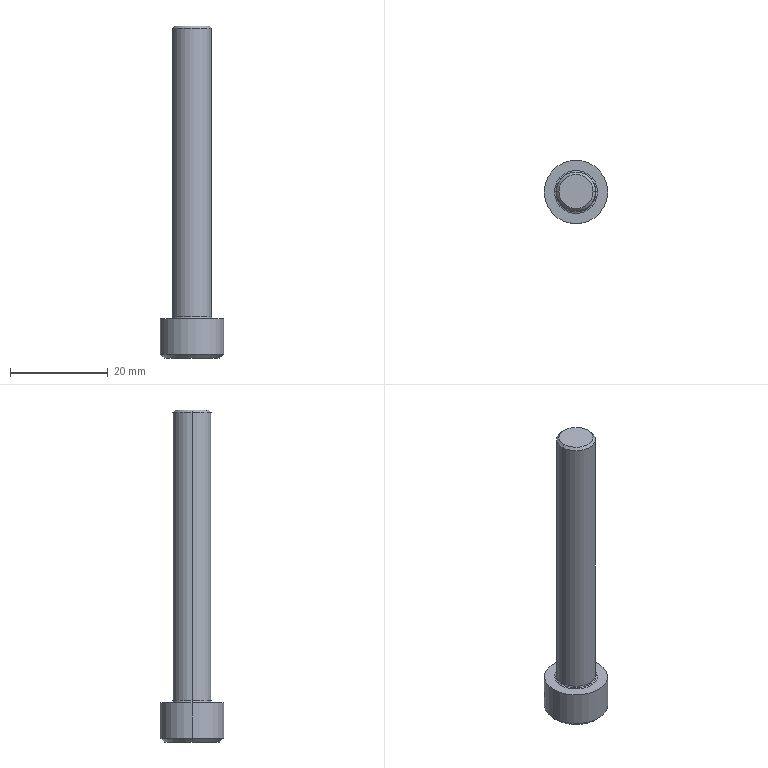Part | Creo | 1 solid | 23 faces | box 13 x 13 x 68 mm | volume 3914 mm3 | plane 9 | cone 6 | cylinder 4 | torus 4 | commonest cylinder face diameters 8 x2 13 x2
STEP:
#1=CARTESIAN_POINT('',(-29.464,-43.932,-100.));
#2=VERTEX_POINT('',#1);
#3=CARTESIAN_POINT('',(-27.732,-40.932,-100.));
#4=VERTEX_POINT('',#3);
#5=CARTESIAN_POINT('',(-29.464,-43.932,-100.));
#6=CARTESIAN_POINT('',(-29.409,-43.836,-99.968));
#7=CARTESIAN_POINT('',(-29.3,-43.647,-99.91));
#8=CARTESIAN_POINT('',(-29.143,-43.375,-99.84));
#9=CARTESIAN_POINT('',(-28.988,-43.108,-99.787));
#10=CARTESIAN_POINT('',(-28.834,-42.84,-99.75));
#11=CARTESIAN_POINT('',(-28.677,-42.568,-99.731));
#12=CARTESIAN_POINT('',(-28.519,-42.295,-99.731));
#13=CARTESIAN_POINT('',(-28.362,-42.023,-99.75));
#14=CARTESIAN_POINT('',(-28.208,-41.755,-99.787));
#15=CARTESIAN_POINT('',(-28.053,-41.488,-99.84));
#16=CARTESIAN_POINT('',(-27.896,-41.216,-99.91));
#17=CARTESIAN_POINT('',(-27.787,-41.027,-99.968));
#18=CARTESIAN_POINT('',(-27.732,-40.932,-100.));
#19=B_SPLINE_CURVE_WITH_KNOTS('',3,(#5,#6,#7,#8,#9,#10,#11,#12,#13,#14,#15,#16,#17,#18),.UNSPECIFIED.,.F.,.F.,(4,1,1,1,1,1,1,1,1,1,1,4),(0.,0.09091,0.1818,0.2727,0.3636,0.4545,0.5455,0.6364,0.7273,0.8182,0.9091,1.),.UNSPECIFIED.);
#20=EDGE_CURVE('',#2,#4,#19,.T.);
#21=ORIENTED_EDGE('',*,*,#20,.F.);
#22=CARTESIAN_POINT('',(-26.,-43.932,-98.));
#23=VERTEX_POINT('',#22);
#24=CARTESIAN_POINT('',(-26.,-43.932,-98.));
#25=DIRECTION('',(-0.866,0.,-0.5));
#26=VECTOR('',#25,4.);
#27=LINE('',#24,#26);
#28=EDGE_CURVE('',#23,#2,#27,.T.);
#29=ORIENTED_EDGE('',*,*,#28,.F.);
#30=CARTESIAN_POINT('',(-22.536,-43.932,-100.));
#31=VERTEX_POINT('',#30);
#32=CARTESIAN_POINT('',(-26.,-43.932,-98.));
#33=DIRECTION('',(0.866,0.,-0.5));
#34=VECTOR('',#33,4.);
#35=LINE('',#32,#34);
#36=EDGE_CURVE('',#23,#31,#35,.T.);
#37=ORIENTED_EDGE('',*,*,#36,.T.);
#38=CARTESIAN_POINT('',(-24.268,-40.932,-100.));
#39=VERTEX_POINT('',#38);
#40=CARTESIAN_POINT('',(-24.268,-40.932,-100.));
#41=CARTESIAN_POINT('',(-24.213,-41.027,-99.968));
#42=CARTESIAN_POINT('',(-24.104,-41.216,-99.91));
#43=CARTESIAN_POINT('',(-23.947,-41.488,-99.84));
#44=CARTESIAN_POINT('',(-23.792,-41.755,-99.787));
#45=CARTESIAN_POINT('',(-23.638,-42.023,-99.75));
#46=CARTESIAN_POINT('',(-23.481,-42.295,-99.731));
#47=CARTESIAN_POINT('',(-23.323,-42.568,-99.731));
#48=CARTESIAN_POINT('',(-23.166,-42.84,-99.75));
#49=CARTESIAN_POINT('',(-23.012,-43.108,-99.787));
#50=CARTESIAN_POINT('',(-22.857,-43.375,-99.84));
#51=CARTESIAN_POINT('',(-22.7,-43.647,-99.91));
#52=CARTESIAN_POINT('',(-22.591,-43.836,-99.968));
#53=CARTESIAN_POINT('',(-22.536,-43.932,-100.));
#54=B_SPLINE_CURVE_WITH_KNOTS('',3,(#40,#41,#42,#43,#44,#45,#46,#47,#48,#49,#50,#51,#52,#53),.UNSPECIFIED.,.F.,.F.,(4,1,1,1,1,1,1,1,1,1,1,4),(0.,0.09091,0.1818,0.2727,0.3636,0.4545,0.5455,0.6364,0.7273,0.8182,0.9091,1.),.UNSPECIFIED.);
#55=EDGE_CURVE('',#39,#31,#54,.T.);
#56=ORIENTED_EDGE('',*,*,#55,.F.);
#57=CARTESIAN_POINT('',(-27.732,-40.932,-100.));
#58=CARTESIAN_POINT('',(-27.622,-40.932,-99.968));
#59=CARTESIAN_POINT('',(-27.404,-40.932,-99.91));
#60=CARTESIAN_POINT('',(-27.091,-40.932,-99.84));
#61=CARTESIAN_POINT('',(-26.782,-40.932,-99.787));
#62=CARTESIAN_POINT('',(-26.472,-40.932,-99.75));
#63=CARTESIAN_POINT('',(-26.158,-40.932,-99.731));
#64=CARTESIAN_POINT('',(-25.842,-40.932,-99.731));
#65=CARTESIAN_POINT('',(-25.528,-40.932,-99.75));
#66=CARTESIAN_POINT('',(-25.218,-40.932,-99.787));
#67=CARTESIAN_POINT('',(-24.909,-40.932,-99.84));
#68=CARTESIAN_POINT('',(-24.596,-40.932,-99.91));
#69=CARTESIAN_POINT('',(-24.378,-40.932,-99.968));
#70=CARTESIAN_POINT('',(-24.268,-40.932,-100.));
#71=B_SPLINE_CURVE_WITH_KNOTS('',3,(#57,#58,#59,#60,#61,#62,#63,#64,#65,#66,#67,#68,#69,#70),.UNSPECIFIED.,.F.,.F.,(4,1,1,1,1,1,1,1,1,1,1,4),(0.,0.09091,0.1818,0.2727,0.3636,0.4545,0.5455,0.6364,0.7273,0.8182,0.9091,1.),.UNSPECIFIED.);
#72=EDGE_CURVE('',#4,#39,#71,.T.);
#73=ORIENTED_EDGE('',*,*,#72,.F.);
#74=EDGE_LOOP('',(#21,#29,#37,#56,#73));
#75=FACE_OUTER_BOUND('',#74,.F.);
#76=CARTESIAN_POINT('',(-26.,-43.932,-99.021));
#77=DIRECTION('',(0.,0.,-1.));
#78=DIRECTION('',(-1.,0.,0.));
#79=AXIS2_PLACEMENT_3D('',#76,#77,#78);
#80=CONICAL_SURFACE('',#79,1.769,60.);
#81=ADVANCED_FACE('',(#75),#80,.F.);
#82=CARTESIAN_POINT('',(-27.732,-40.932,-104.));
#83=VERTEX_POINT('',#82);
#84=CARTESIAN_POINT('',(-29.464,-43.932,-104.));
#85=VERTEX_POINT('',#84);
#86=CARTESIAN_POINT('',(-27.732,-40.932,-104.));
#87=DIRECTION('',(-0.5,-0.866,0.));
#88=VECTOR('',#87,3.464);
#89=LINE('',#86,#88);
#90=EDGE_CURVE('',#83,#85,#89,.T.);
#91=ORIENTED_EDGE('',*,*,#90,.T.);
#92=CARTESIAN_POINT('',(-29.464,-43.932,-104.));
#93=DIRECTION('',(0.,0.,1.));
#94=VECTOR('',#93,4.);
#95=LINE('',#92,#94);
#96=EDGE_CURVE('',#85,#2,#95,.T.);
#97=ORIENTED_EDGE('',*,*,#96,.T.);
#98=ORIENTED_EDGE('',*,*,#20,.T.);
#99=CARTESIAN_POINT('',(-27.732,-40.932,-104.));
#100=DIRECTION('',(0.,0.,1.));
#101=VECTOR('',#100,4.);
#102=LINE('',#99,#101);
#103=EDGE_CURVE('',#83,#4,#102,.T.);
#104=ORIENTED_EDGE('',*,*,#103,.F.);
#105=EDGE_LOOP('',(#91,#97,#98,#104));
#106=FACE_OUTER_BOUND('',#105,.F.);
#107=CARTESIAN_POINT('',(-27.732,-40.932,-100.));
#108=DIRECTION('',(0.866,-0.5,0.));
#109=DIRECTION('',(-0.5,-0.866,0.));
#110=AXIS2_PLACEMENT_3D('',#107,#108,#109);
#111=PLANE('',#110);
#112=ADVANCED_FACE('',(#106),#111,.T.);
#113=CARTESIAN_POINT('',(-31.7,-43.932,-104.));
#114=VERTEX_POINT('',#113);
#115=CARTESIAN_POINT('',(-20.3,-43.932,-104.));
#116=VERTEX_POINT('',#115);
#117=CARTESIAN_POINT('',(-26.,-43.932,-104.));
#118=DIRECTION('',(0.,0.,-1.));
#119=DIRECTION('',(-1.,0.,0.));
#120=AXIS2_PLACEMENT_3D('',#117,#118,#119);
#121=CIRCLE('',#120,5.7);
#122=EDGE_CURVE('',#114,#116,#121,.T.);
#123=ORIENTED_EDGE('',*,*,#122,.F.);
#124=CARTESIAN_POINT('',(-26.,-43.932,-104.));
#125=DIRECTION('',(0.,0.,-1.));
#126=DIRECTION('',(1.,0.,0.));
#127=AXIS2_PLACEMENT_3D('',#124,#125,#126);
#128=CIRCLE('',#127,5.7);
#129=EDGE_CURVE('',#116,#114,#128,.T.);
#130=ORIENTED_EDGE('',*,*,#129,.F.);
#131=EDGE_LOOP('',(#123,#130));
#132=FACE_OUTER_BOUND('',#131,.F.);
#133=CARTESIAN_POINT('',(-27.732,-46.932,-104.));
#134=VERTEX_POINT('',#133);
#135=CARTESIAN_POINT('',(-29.464,-43.932,-104.));
#136=DIRECTION('',(0.5,-0.866,0.));
#137=VECTOR('',#136,3.464);
#138=LINE('',#135,#137);
#139=EDGE_CURVE('',#85,#134,#138,.T.);
#140=ORIENTED_EDGE('',*,*,#139,.F.);
#141=ORIENTED_EDGE('',*,*,#90,.F.);
#142=CARTESIAN_POINT('',(-24.268,-40.932,-104.));
#143=VERTEX_POINT('',#142);
#144=CARTESIAN_POINT('',(-27.732,-40.932,-104.));
#145=DIRECTION('',(1.,0.,0.));
#146=VECTOR('',#145,3.464);
#147=LINE('',#144,#146);
#148=EDGE_CURVE('',#83,#143,#147,.T.);
#149=ORIENTED_EDGE('',*,*,#148,.T.);
#150=CARTESIAN_POINT('',(-22.536,-43.932,-104.));
#151=VERTEX_POINT('',#150);
#152=CARTESIAN_POINT('',(-22.536,-43.932,-104.));
#153=DIRECTION('',(-0.5,0.866,0.));
#154=VECTOR('',#153,3.464);
#155=LINE('',#152,#154);
#156=EDGE_CURVE('',#151,#143,#155,.T.);
#157=ORIENTED_EDGE('',*,*,#156,.F.);
#158=CARTESIAN_POINT('',(-24.268,-46.932,-104.));
#159=VERTEX_POINT('',#158);
#160=CARTESIAN_POINT('',(-24.268,-46.932,-104.));
#161=DIRECTION('',(0.5,0.866,0.));
#162=VECTOR('',#161,3.464);
#163=LINE('',#160,#162);
#164=EDGE_CURVE('',#159,#151,#163,.T.);
#165=ORIENTED_EDGE('',*,*,#164,.F.);
#166=CARTESIAN_POINT('',(-24.268,-46.932,-104.));
#167=DIRECTION('',(-1.,0.,0.));
#168=VECTOR('',#167,3.464);
#169=LINE('',#166,#168);
#170=EDGE_CURVE('',#159,#134,#169,.T.);
#171=ORIENTED_EDGE('',*,*,#170,.T.);
#172=EDGE_LOOP('',(#140,#141,#149,#157,#165,#171));
#173=FACE_BOUND('',#172,.F.);
#174=CARTESIAN_POINT('',(-26.,-43.932,-104.));
#175=DIRECTION('',(0.,0.,-1.));
#176=DIRECTION('',(-1.,0.,0.));
#177=AXIS2_PLACEMENT_3D('',#174,#175,#176);
#178=PLANE('',#177);
#179=ADVANCED_FACE('',(#132,#173),#178,.T.);
#180=CARTESIAN_POINT('',(-32.5,-43.932,-103.2));
#181=VERTEX_POINT('',#180);
#182=CARTESIAN_POINT('',(-19.5,-43.932,-103.2));
#183=VERTEX_POINT('',#182);
#184=CARTESIAN_POINT('',(-26.,-43.932,-103.2));
#185=DIRECTION('',(0.,0.,-1.));
#186=DIRECTION('',(-1.,0.,0.));
#187=AXIS2_PLACEMENT_3D('',#184,#185,#186);
#188=CIRCLE('',#187,6.5);
#189=EDGE_CURVE('',#181,#183,#188,.T.);
#190=ORIENTED_EDGE('',*,*,#189,.F.);
#191=CARTESIAN_POINT('',(-31.7,-43.932,-104.));
#192=DIRECTION('',(-0.7071,0.,0.7071));
#193=VECTOR('',#192,1.131);
#194=LINE('',#191,#193);
#195=EDGE_CURVE('',#114,#181,#194,.T.);
#196=ORIENTED_EDGE('',*,*,#195,.F.);
#197=ORIENTED_EDGE('',*,*,#122,.T.);
#198=CARTESIAN_POINT('',(-20.3,-43.932,-104.));
#199=DIRECTION('',(0.7071,0.,0.7071));
#200=VECTOR('',#199,1.131);
#201=LINE('',#198,#200);
#202=EDGE_CURVE('',#116,#183,#201,.T.);
#203=ORIENTED_EDGE('',*,*,#202,.T.);
#204=EDGE_LOOP('',(#190,#196,#197,#203));
#205=FACE_OUTER_BOUND('',#204,.F.);
#206=CARTESIAN_POINT('',(-26.,-43.932,-103.6));
#207=DIRECTION('',(0.,0.,1.));
#208=DIRECTION('',(1.,0.,0.));
#209=AXIS2_PLACEMENT_3D('',#206,#207,#208);
#210=CONICAL_SURFACE('',#209,6.1,45.);
#211=ADVANCED_FACE('',(#205),#210,.T.);
#212=ORIENTED_EDGE('',*,*,#189,.T.);
#213=CARTESIAN_POINT('',(-19.5,-43.932,-96.));
#214=VERTEX_POINT('',#213);
#215=CARTESIAN_POINT('',(-19.5,-43.932,-96.));
#216=DIRECTION('',(0.,0.,-1.));
#217=VECTOR('',#216,7.2);
#218=LINE('',#215,#217);
#219=EDGE_CURVE('',#214,#183,#218,.T.);
#220=ORIENTED_EDGE('',*,*,#219,.F.);
#221=CARTESIAN_POINT('',(-32.5,-43.932,-96.));
#222=VERTEX_POINT('',#221);
#223=CARTESIAN_POINT('',(-26.,-43.932,-96.));
#224=DIRECTION('',(0.,0.,1.));
#225=DIRECTION('',(1.,0.,0.));
#226=AXIS2_PLACEMENT_3D('',#223,#224,#225);
#227=CIRCLE('',#226,6.5);
#228=EDGE_CURVE('',#214,#222,#227,.T.);
#229=ORIENTED_EDGE('',*,*,#228,.T.);
#230=CARTESIAN_POINT('',(-32.5,-43.932,-96.));
#231=DIRECTION('',(0.,0.,-1.));
#232=VECTOR('',#231,7.2);
#233=LINE('',#230,#232);
#234=EDGE_CURVE('',#222,#181,#233,.T.);
#235=ORIENTED_EDGE('',*,*,#234,.T.);
#236=EDGE_LOOP('',(#212,#220,#229,#235));
#237=FACE_OUTER_BOUND('',#236,.F.);
#238=CARTESIAN_POINT('',(-26.,-43.932,-96.));
#239=DIRECTION('',(0.,0.,-1.));
#240=DIRECTION('',(-1.,0.,0.));
#241=AXIS2_PLACEMENT_3D('',#238,#239,#240);
#242=CYLINDRICAL_SURFACE('',#241,6.5);
#243=ADVANCED_FACE('',(#237),#242,.T.);
#244=CARTESIAN_POINT('',(-26.,-43.932,-103.2));
#245=DIRECTION('',(0.,0.,-1.));
#246=DIRECTION('',(1.,0.,0.));
#247=AXIS2_PLACEMENT_3D('',#244,#245,#246);
#248=CIRCLE('',#247,6.5);
#249=EDGE_CURVE('',#183,#181,#248,.T.);
#250=ORIENTED_EDGE('',*,*,#249,.T.);
#251=ORIENTED_EDGE('',*,*,#234,.F.);
#252=CARTESIAN_POINT('',(-26.,-43.932,-96.));
#253=DIRECTION('',(0.,0.,1.));
#254=DIRECTION('',(-1.,0.,0.));
#255=AXIS2_PLACEMENT_3D('',#252,#253,#254);
#256=CIRCLE('',#255,6.5);
#257=EDGE_CURVE('',#222,#214,#256,.T.);
#258=ORIENTED_EDGE('',*,*,#257,.T.);
#259=ORIENTED_EDGE('',*,*,#219,.T.);
#260=EDGE_LOOP('',(#250,#251,#258,#259));
#261=FACE_OUTER_BOUND('',#260,.F.);
#262=CARTESIAN_POINT('',(-26.,-43.932,-96.));
#263=DIRECTION('',(0.,0.,-1.));
#264=DIRECTION('',(-1.,0.,0.));
#265=AXIS2_PLACEMENT_3D('',#262,#263,#264);
#266=CYLINDRICAL_SURFACE('',#265,6.5);
#267=ADVANCED_FACE('',(#261),#266,.T.);
#268=ORIENTED_EDGE('',*,*,#249,.F.);
#269=ORIENTED_EDGE('',*,*,#202,.F.);
#270=ORIENTED_EDGE('',*,*,#129,.T.);
#271=ORIENTED_EDGE('',*,*,#195,.T.);
#272=EDGE_LOOP('',(#268,#269,#270,#271));
#273=FACE_OUTER_BOUND('',#272,.F.);
#274=CARTESIAN_POINT('',(-26.,-43.932,-103.6));
#275=DIRECTION('',(0.,0.,1.));
#276=DIRECTION('',(1.,0.,0.));
#277=AXIS2_PLACEMENT_3D('',#274,#275,#276);
#278=CONICAL_SURFACE('',#277,6.1,45.);
#279=ADVANCED_FACE('',(#273),#278,.T.);
#280=ORIENTED_EDGE('',*,*,#257,.F.);
#281=ORIENTED_EDGE('',*,*,#228,.F.);
#282=EDGE_LOOP('',(#280,#281));
#283=FACE_OUTER_BOUND('',#282,.F.);
#284=CARTESIAN_POINT('',(-30.4,-43.932,-96.));
#285=VERTEX_POINT('',#284);
#286=CARTESIAN_POINT('',(-21.6,-43.932,-96.));
#287=VERTEX_POINT('',#286);
#288=CARTESIAN_POINT('',(-26.,-43.932,-96.));
#289=DIRECTION('',(0.,0.,-1.));
#290=DIRECTION('',(-1.,0.,0.));
#291=AXIS2_PLACEMENT_3D('',#288,#289,#290);
#292=CIRCLE('',#291,4.4);
#293=EDGE_CURVE('',#285,#287,#292,.T.);
#294=ORIENTED_EDGE('',*,*,#293,.F.);
#295=CARTESIAN_POINT('',(-26.,-43.932,-96.));
#296=DIRECTION('',(0.,0.,-1.));
#297=DIRECTION('',(1.,0.,0.));
#298=AXIS2_PLACEMENT_3D('',#295,#296,#297);
#299=CIRCLE('',#298,4.4);
#300=EDGE_CURVE('',#287,#285,#299,.T.);
#301=ORIENTED_EDGE('',*,*,#300,.F.);
#302=EDGE_LOOP('',(#294,#301));
#303=FACE_BOUND('',#302,.F.);
#304=CARTESIAN_POINT('',(-26.,-43.932,-96.));
#305=DIRECTION('',(0.,0.,-1.));
#306=DIRECTION('',(-1.,0.,0.));
#307=AXIS2_PLACEMENT_3D('',#304,#305,#306);
#308=PLANE('',#307);
#309=ADVANCED_FACE('',(#283,#303),#308,.F.);
#310=ORIENTED_EDGE('',*,*,#293,.T.);
#311=CARTESIAN_POINT('',(-21.883,-43.932,-95.883));
#312=VERTEX_POINT('',#311);
#313=CARTESIAN_POINT('',(-21.6,-43.932,-95.6));
#314=DIRECTION('',(0.,1.,0.));
#315=DIRECTION('',(0.,0.,-1.));
#316=AXIS2_PLACEMENT_3D('',#313,#314,#315);
#317=CIRCLE('',#316,0.4);
#318=EDGE_CURVE('',#287,#312,#317,.T.);
#319=ORIENTED_EDGE('',*,*,#318,.T.);
#320=CARTESIAN_POINT('',(-30.117,-43.932,-95.883));
#321=VERTEX_POINT('',#320);
#322=CARTESIAN_POINT('',(-26.,-43.932,-95.883));
#323=DIRECTION('',(0.,0.,-1.));
#324=DIRECTION('',(-1.,0.,0.));
#325=AXIS2_PLACEMENT_3D('',#322,#323,#324);
#326=CIRCLE('',#325,4.117);
#327=EDGE_CURVE('',#321,#312,#326,.T.);
#328=ORIENTED_EDGE('',*,*,#327,.F.);
#329=CARTESIAN_POINT('',(-30.4,-43.932,-95.6));
#330=DIRECTION('',(0.,-1.,0.));
#331=DIRECTION('',(0.,0.,-1.));
#332=AXIS2_PLACEMENT_3D('',#329,#330,#331);
#333=CIRCLE('',#332,0.4);
#334=EDGE_CURVE('',#285,#321,#333,.T.);
#335=ORIENTED_EDGE('',*,*,#334,.F.);
#336=EDGE_LOOP('',(#310,#319,#328,#335));
#337=FACE_OUTER_BOUND('',#336,.F.);
#338=CARTESIAN_POINT('',(-26.,-43.932,-95.6));
#339=DIRECTION('',(0.,0.,-1.));
#340=DIRECTION('',(-1.,0.,0.));
#341=AXIS2_PLACEMENT_3D('',#338,#339,#340);
#342=TOROIDAL_SURFACE('',#341,4.4,0.4);
#343=ADVANCED_FACE('',(#337),#342,.F.);
#344=ORIENTED_EDGE('',*,*,#300,.T.);
#345=ORIENTED_EDGE('',*,*,#334,.T.);
#346=CARTESIAN_POINT('',(-26.,-43.932,-95.883));
#347=DIRECTION('',(0.,0.,-1.));
#348=DIRECTION('',(1.,0.,0.));
#349=AXIS2_PLACEMENT_3D('',#346,#347,#348);
#350=CIRCLE('',#349,4.117);
#351=EDGE_CURVE('',#312,#321,#350,.T.);
#352=ORIENTED_EDGE('',*,*,#351,.F.);
#353=ORIENTED_EDGE('',*,*,#318,.F.);
#354=EDGE_LOOP('',(#344,#345,#352,#353));
#355=FACE_OUTER_BOUND('',#354,.F.);
#356=CARTESIAN_POINT('',(-26.,-43.932,-95.6));
#357=DIRECTION('',(0.,0.,-1.));
#358=DIRECTION('',(-1.,0.,0.));
#359=AXIS2_PLACEMENT_3D('',#356,#357,#358);
#360=TOROIDAL_SURFACE('',#359,4.4,0.4);
#361=ADVANCED_FACE('',(#355),#360,.F.);
#362=CARTESIAN_POINT('',(-22.,-43.932,-95.6));
#363=VERTEX_POINT('',#362);
#364=CARTESIAN_POINT('',(-30.,-43.932,-95.6));
#365=VERTEX_POINT('',#364);
#366=CARTESIAN_POINT('',(-26.,-43.932,-95.6));
#367=DIRECTION('',(0.,0.,-1.));
#368=DIRECTION('',(1.,0.,0.));
#369=AXIS2_PLACEMENT_3D('',#366,#367,#368);
#370=CIRCLE('',#369,4.);
#371=EDGE_CURVE('',#363,#365,#370,.T.);
#372=ORIENTED_EDGE('',*,*,#371,.F.);
#373=CARTESIAN_POINT('',(-21.6,-43.932,-95.6));
#374=DIRECTION('',(0.,1.,0.));
#375=DIRECTION('',(-0.7071,0.,-0.7071));
#376=AXIS2_PLACEMENT_3D('',#373,#374,#375);
#377=CIRCLE('',#376,0.4);
#378=EDGE_CURVE('',#312,#363,#377,.T.);
#379=ORIENTED_EDGE('',*,*,#378,.F.);
#380=ORIENTED_EDGE('',*,*,#351,.T.);
#381=CARTESIAN_POINT('',(-30.4,-43.932,-95.6));
#382=DIRECTION('',(0.,-1.,0.));
#383=DIRECTION('',(0.7071,0.,-0.7071));
#384=AXIS2_PLACEMENT_3D('',#381,#382,#383);
#385=CIRCLE('',#384,0.4);
#386=EDGE_CURVE('',#321,#365,#385,.T.);
#387=ORIENTED_EDGE('',*,*,#386,.T.);
#388=EDGE_LOOP('',(#372,#379,#380,#387));
#389=FACE_OUTER_BOUND('',#388,.F.);
#390=CARTESIAN_POINT('',(-26.,-43.932,-95.6));
#391=DIRECTION('',(0.,0.,-1.));
#392=DIRECTION('',(-1.,0.,0.));
#393=AXIS2_PLACEMENT_3D('',#390,#391,#392);
#394=TOROIDAL_SURFACE('',#393,4.4,0.4);
#395=ADVANCED_FACE('',(#389),#394,.F.);
#396=CARTESIAN_POINT('',(-30.,-43.932,-36.5));
#397=VERTEX_POINT('',#396);
#398=CARTESIAN_POINT('',(-22.,-43.932,-36.5));
#399=VERTEX_POINT('',#398);
#400=CARTESIAN_POINT('',(-26.,-43.932,-36.5));
#401=DIRECTION('',(0.,0.,1.));
#402=DIRECTION('',(-1.,0.,0.));
#403=AXIS2_PLACEMENT_3D('',#400,#401,#402);
#404=CIRCLE('',#403,4.);
#405=EDGE_CURVE('',#397,#399,#404,.T.);
#406=ORIENTED_EDGE('',*,*,#405,.T.);
#407=CARTESIAN_POINT('',(-22.,-43.932,-36.5));
#408=DIRECTION('',(0.,0.,-1.));
#409=VECTOR('',#408,59.1);
#410=LINE('',#407,#409);
#411=EDGE_CURVE('',#399,#363,#410,.T.);
#412=ORIENTED_EDGE('',*,*,#411,.T.);
#413=ORIENTED_EDGE('',*,*,#371,.T.);
#414=CARTESIAN_POINT('',(-30.,-43.932,-36.5));
#415=DIRECTION('',(0.,0.,-1.));
#416=VECTOR('',#415,59.1);
#417=LINE('',#414,#416);
#418=EDGE_CURVE('',#397,#365,#417,.T.);
#419=ORIENTED_EDGE('',*,*,#418,.F.);
#420=EDGE_LOOP('',(#406,#412,#413,#419));
#421=FACE_OUTER_BOUND('',#420,.F.);
#422=CARTESIAN_POINT('',(-26.,-43.932,-36.));
#423=DIRECTION('',(0.,0.,-1.));
#424=DIRECTION('',(-1.,0.,0.));
#425=AXIS2_PLACEMENT_3D('',#422,#423,#424);
#426=CYLINDRICAL_SURFACE('',#425,4.);
#427=ADVANCED_FACE('',(#421),#426,.T.);
#428=CARTESIAN_POINT('',(-29.5,-43.932,-36.));
#429=VERTEX_POINT('',#428);
#430=CARTESIAN_POINT('',(-22.5,-43.932,-36.));
#431=VERTEX_POINT('',#430);
#432=CARTESIAN_POINT('',(-26.,-43.932,-36.));
#433=DIRECTION('',(0.,0.,1.));
#434=DIRECTION('',(-1.,0.,0.));
#435=AXIS2_PLACEMENT_3D('',#432,#433,#434);
#436=CIRCLE('',#435,3.5);
#437=EDGE_CURVE('',#429,#431,#436,.T.);
#438=ORIENTED_EDGE('',*,*,#437,.T.);
#439=CARTESIAN_POINT('',(-22.5,-43.932,-36.));
#440=DIRECTION('',(0.7071,0.,-0.7071));
#441=VECTOR('',#440,0.7071);
#442=LINE('',#439,#441);
#443=EDGE_CURVE('',#431,#399,#442,.T.);
#444=ORIENTED_EDGE('',*,*,#443,.T.);
#445=ORIENTED_EDGE('',*,*,#405,.F.);
#446=CARTESIAN_POINT('',(-29.5,-43.932,-36.));
#447=DIRECTION('',(-0.7071,0.,-0.7071));
#448=VECTOR('',#447,0.7071);
#449=LINE('',#446,#448);
#450=EDGE_CURVE('',#429,#397,#449,.T.);
#451=ORIENTED_EDGE('',*,*,#450,.F.);
#452=EDGE_LOOP('',(#438,#444,#445,#451));
#453=FACE_OUTER_BOUND('',#452,.F.);
#454=CARTESIAN_POINT('',(-26.,-43.932,-36.25));
#455=DIRECTION('',(0.,0.,-1.));
#456=DIRECTION('',(-1.,0.,0.));
#457=AXIS2_PLACEMENT_3D('',#454,#455,#456);
#458=CONICAL_SURFACE('',#457,3.75,45.);
#459=ADVANCED_FACE('',(#453),#458,.T.);
#460=ORIENTED_EDGE('',*,*,#437,.F.);
#461=CARTESIAN_POINT('',(-26.,-43.932,-36.));
#462=DIRECTION('',(0.,0.,1.));
#463=DIRECTION('',(1.,0.,0.));
#464=AXIS2_PLACEMENT_3D('',#461,#462,#463);
#465=CIRCLE('',#464,3.5);
#466=EDGE_CURVE('',#431,#429,#465,.T.);
#467=ORIENTED_EDGE('',*,*,#466,.F.);
#468=EDGE_LOOP('',(#460,#467));
#469=FACE_OUTER_BOUND('',#468,.F.);
#470=CARTESIAN_POINT('',(-26.,-43.932,-36.));
#471=DIRECTION('',(0.,0.,-1.));
#472=DIRECTION('',(-1.,0.,0.));
#473=AXIS2_PLACEMENT_3D('',#470,#471,#472);
#474=PLANE('',#473);
#475=ADVANCED_FACE('',(#469),#474,.F.);
#476=ORIENTED_EDGE('',*,*,#466,.T.);
#477=ORIENTED_EDGE('',*,*,#450,.T.);
#478=CARTESIAN_POINT('',(-26.,-43.932,-36.5));
#479=DIRECTION('',(0.,0.,1.));
#480=DIRECTION('',(1.,0.,0.));
#481=AXIS2_PLACEMENT_3D('',#478,#479,#480);
#482=CIRCLE('',#481,4.);
#483=EDGE_CURVE('',#399,#397,#482,.T.);
#484=ORIENTED_EDGE('',*,*,#483,.F.);
#485=ORIENTED_EDGE('',*,*,#443,.F.);
#486=EDGE_LOOP('',(#476,#477,#484,#485));
#487=FACE_OUTER_BOUND('',#486,.F.);
#488=CARTESIAN_POINT('',(-26.,-43.932,-36.25));
#489=DIRECTION('',(0.,0.,-1.));
#490=DIRECTION('',(-1.,0.,0.));
#491=AXIS2_PLACEMENT_3D('',#488,#489,#490);
#492=CONICAL_SURFACE('',#491,3.75,45.);
#493=ADVANCED_FACE('',(#487),#492,.T.);
#494=ORIENTED_EDGE('',*,*,#483,.T.);
#495=ORIENTED_EDGE('',*,*,#418,.T.);
#496=CARTESIAN_POINT('',(-26.,-43.932,-95.6));
#497=DIRECTION('',(0.,0.,-1.));
#498=DIRECTION('',(-1.,0.,0.));
#499=AXIS2_PLACEMENT_3D('',#496,#497,#498);
#500=CIRCLE('',#499,4.);
#501=EDGE_CURVE('',#365,#363,#500,.T.);
#502=ORIENTED_EDGE('',*,*,#501,.T.);
#503=ORIENTED_EDGE('',*,*,#411,.F.);
#504=EDGE_LOOP('',(#494,#495,#502,#503));
#505=FACE_OUTER_BOUND('',#504,.F.);
#506=CARTESIAN_POINT('',(-26.,-43.932,-36.));
#507=DIRECTION('',(0.,0.,-1.));
#508=DIRECTION('',(-1.,0.,0.));
#509=AXIS2_PLACEMENT_3D('',#506,#507,#508);
#510=CYLINDRICAL_SURFACE('',#509,4.);
#511=ADVANCED_FACE('',(#505),#510,.T.);
#512=ORIENTED_EDGE('',*,*,#501,.F.);
#513=ORIENTED_EDGE('',*,*,#386,.F.);
#514=ORIENTED_EDGE('',*,*,#327,.T.);
#515=ORIENTED_EDGE('',*,*,#378,.T.);
#516=EDGE_LOOP('',(#512,#513,#514,#515));
#517=FACE_OUTER_BOUND('',#516,.F.);
#518=CARTESIAN_POINT('',(-26.,-43.932,-95.6));
#519=DIRECTION('',(0.,0.,-1.));
#520=DIRECTION('',(-1.,0.,0.));
#521=AXIS2_PLACEMENT_3D('',#518,#519,#520);
#522=TOROIDAL_SURFACE('',#521,4.4,0.4);
#523=ADVANCED_FACE('',(#517),#522,.F.);
#524=ORIENTED_EDGE('',*,*,#139,.T.);
#525=CARTESIAN_POINT('',(-27.732,-46.932,-100.));
#526=VERTEX_POINT('',#525);
#527=CARTESIAN_POINT('',(-27.732,-46.932,-104.));
#528=DIRECTION('',(0.,0.,1.));
#529=VECTOR('',#528,4.);
#530=LINE('',#527,#529);
#531=EDGE_CURVE('',#134,#526,#530,.T.);
#532=ORIENTED_EDGE('',*,*,#531,.T.);
#533=CARTESIAN_POINT('',(-27.732,-46.932,-100.));
#534=CARTESIAN_POINT('',(-27.787,-46.836,-99.968));
#535=CARTESIAN_POINT('',(-27.896,-46.647,-99.91));
#536=CARTESIAN_POINT('',(-28.053,-46.375,-99.84));
#537=CARTESIAN_POINT('',(-28.208,-46.108,-99.787));
#538=CARTESIAN_POINT('',(-28.362,-45.84,-99.75));
#539=CARTESIAN_POINT('',(-28.519,-45.568,-99.731));
#540=CARTESIAN_POINT('',(-28.677,-45.295,-99.731));
#541=CARTESIAN_POINT('',(-28.834,-45.023,-99.75));
#542=CARTESIAN_POINT('',(-28.988,-44.755,-99.787));
#543=CARTESIAN_POINT('',(-29.143,-44.488,-99.84));
#544=CARTESIAN_POINT('',(-29.3,-44.216,-99.91));
#545=CARTESIAN_POINT('',(-29.409,-44.027,-99.968));
#546=CARTESIAN_POINT('',(-29.464,-43.932,-100.));
#547=B_SPLINE_CURVE_WITH_KNOTS('',3,(#533,#534,#535,#536,#537,#538,#539,#540,#541,#542,#543,#544,#545,#546),.UNSPECIFIED.,.F.,.F.,(4,1,1,1,1,1,1,1,1,1,1,4),(0.,0.09091,0.1818,0.2727,0.3636,0.4545,0.5455,0.6364,0.7273,0.8182,0.9091,1.),.UNSPECIFIED.);
#548=EDGE_CURVE('',#526,#2,#547,.T.);
#549=ORIENTED_EDGE('',*,*,#548,.T.);
#550=ORIENTED_EDGE('',*,*,#96,.F.);
#551=EDGE_LOOP('',(#524,#532,#549,#550));
#552=FACE_OUTER_BOUND('',#551,.F.);
#553=CARTESIAN_POINT('',(-29.464,-43.932,-100.));
#554=DIRECTION('',(0.866,0.5,0.));
#555=DIRECTION('',(0.5,-0.866,0.));
#556=AXIS2_PLACEMENT_3D('',#553,#554,#555);
#557=PLANE('',#556);
#558=ADVANCED_FACE('',(#552),#557,.T.);
#559=ORIENTED_EDGE('',*,*,#170,.F.);
#560=CARTESIAN_POINT('',(-24.268,-46.932,-100.));
#561=VERTEX_POINT('',#560);
#562=CARTESIAN_POINT('',(-24.268,-46.932,-104.));
#563=DIRECTION('',(0.,0.,1.));
#564=VECTOR('',#563,4.);
#565=LINE('',#562,#564);
#566=EDGE_CURVE('',#159,#561,#565,.T.);
#567=ORIENTED_EDGE('',*,*,#566,.T.);
#568=CARTESIAN_POINT('',(-24.268,-46.932,-100.));
#569=CARTESIAN_POINT('',(-24.378,-46.932,-99.968));
#570=CARTESIAN_POINT('',(-24.596,-46.932,-99.91));
#571=CARTESIAN_POINT('',(-24.909,-46.932,-99.84));
#572=CARTESIAN_POINT('',(-25.218,-46.932,-99.787));
#573=CARTESIAN_POINT('',(-25.528,-46.932,-99.75));
#574=CARTESIAN_POINT('',(-25.842,-46.932,-99.731));
#575=CARTESIAN_POINT('',(-26.158,-46.932,-99.731));
#576=CARTESIAN_POINT('',(-26.472,-46.932,-99.75));
#577=CARTESIAN_POINT('',(-26.782,-46.932,-99.787));
#578=CARTESIAN_POINT('',(-27.091,-46.932,-99.84));
#579=CARTESIAN_POINT('',(-27.404,-46.932,-99.91));
#580=CARTESIAN_POINT('',(-27.622,-46.932,-99.968));
#581=CARTESIAN_POINT('',(-27.732,-46.932,-100.));
#582=B_SPLINE_CURVE_WITH_KNOTS('',3,(#568,#569,#570,#571,#572,#573,#574,#575,#576,#577,#578,#579,#580,#581),.UNSPECIFIED.,.F.,.F.,(4,1,1,1,1,1,1,1,1,1,1,4),(0.,0.09091,0.1818,0.2727,0.3636,0.4545,0.5455,0.6364,0.7273,0.8182,0.9091,1.),.UNSPECIFIED.);
#583=EDGE_CURVE('',#561,#526,#582,.T.);
#584=ORIENTED_EDGE('',*,*,#583,.T.);
#585=ORIENTED_EDGE('',*,*,#531,.F.);
#586=EDGE_LOOP('',(#559,#567,#584,#585));
#587=FACE_OUTER_BOUND('',#586,.F.);
#588=CARTESIAN_POINT('',(-27.732,-46.932,-100.));
#589=DIRECTION('',(0.,1.,0.));
#590=DIRECTION('',(0.,0.,-1.));
#591=AXIS2_PLACEMENT_3D('',#588,#589,#590);
#592=PLANE('',#591);
#593=ADVANCED_FACE('',(#587),#592,.T.);
#594=ORIENTED_EDGE('',*,*,#164,.T.);
#595=CARTESIAN_POINT('',(-22.536,-43.932,-104.));
#596=DIRECTION('',(0.,0.,1.));
#597=VECTOR('',#596,4.);
#598=LINE('',#595,#597);
#599=EDGE_CURVE('',#151,#31,#598,.T.);
#600=ORIENTED_EDGE('',*,*,#599,.T.);
#601=CARTESIAN_POINT('',(-22.536,-43.932,-100.));
#602=CARTESIAN_POINT('',(-22.591,-44.027,-99.968));
#603=CARTESIAN_POINT('',(-22.7,-44.216,-99.91));
#604=CARTESIAN_POINT('',(-22.857,-44.488,-99.84));
#605=CARTESIAN_POINT('',(-23.012,-44.755,-99.787));
#606=CARTESIAN_POINT('',(-23.166,-45.023,-99.75));
#607=CARTESIAN_POINT('',(-23.323,-45.295,-99.731));
#608=CARTESIAN_POINT('',(-23.481,-45.568,-99.731));
#609=CARTESIAN_POINT('',(-23.638,-45.84,-99.75));
#610=CARTESIAN_POINT('',(-23.792,-46.108,-99.787));
#611=CARTESIAN_POINT('',(-23.947,-46.375,-99.84));
#612=CARTESIAN_POINT('',(-24.104,-46.647,-99.91));
#613=CARTESIAN_POINT('',(-24.213,-46.836,-99.968));
#614=CARTESIAN_POINT('',(-24.268,-46.932,-100.));
#615=B_SPLINE_CURVE_WITH_KNOTS('',3,(#601,#602,#603,#604,#605,#606,#607,#608,#609,#610,#611,#612,#613,#614),.UNSPECIFIED.,.F.,.F.,(4,1,1,1,1,1,1,1,1,1,1,4),(0.,0.09091,0.1818,0.2727,0.3636,0.4545,0.5455,0.6364,0.7273,0.8182,0.9091,1.),.UNSPECIFIED.);
#616=EDGE_CURVE('',#31,#561,#615,.T.);
#617=ORIENTED_EDGE('',*,*,#616,.T.);
#618=ORIENTED_EDGE('',*,*,#566,.F.);
#619=EDGE_LOOP('',(#594,#600,#617,#618));
#620=FACE_OUTER_BOUND('',#619,.F.);
#621=CARTESIAN_POINT('',(-24.268,-46.932,-100.));
#622=DIRECTION('',(-0.866,0.5,0.));
#623=DIRECTION('',(0.5,0.866,0.));
#624=AXIS2_PLACEMENT_3D('',#621,#622,#623);
#625=PLANE('',#624);
#626=ADVANCED_FACE('',(#620),#625,.T.);
#627=ORIENTED_EDGE('',*,*,#156,.T.);
#628=CARTESIAN_POINT('',(-24.268,-40.932,-104.));
#629=DIRECTION('',(0.,0.,1.));
#630=VECTOR('',#629,4.);
#631=LINE('',#628,#630);
#632=EDGE_CURVE('',#143,#39,#631,.T.);
#633=ORIENTED_EDGE('',*,*,#632,.T.);
#634=ORIENTED_EDGE('',*,*,#55,.T.);
#635=ORIENTED_EDGE('',*,*,#599,.F.);
#636=EDGE_LOOP('',(#627,#633,#634,#635));
#637=FACE_OUTER_BOUND('',#636,.F.);
#638=CARTESIAN_POINT('',(-22.536,-43.932,-100.));
#639=DIRECTION('',(-0.866,-0.5,0.));
#640=DIRECTION('',(-0.5,0.866,0.));
#641=AXIS2_PLACEMENT_3D('',#638,#639,#640);
#642=PLANE('',#641);
#643=ADVANCED_FACE('',(#637),#642,.T.);
#644=ORIENTED_EDGE('',*,*,#148,.F.);
#645=ORIENTED_EDGE('',*,*,#103,.T.);
#646=ORIENTED_EDGE('',*,*,#72,.T.);
#647=ORIENTED_EDGE('',*,*,#632,.F.);
#648=EDGE_LOOP('',(#644,#645,#646,#647));
#649=FACE_OUTER_BOUND('',#648,.F.);
#650=CARTESIAN_POINT('',(-24.268,-40.932,-100.));
#651=DIRECTION('',(0.,-1.,0.));
#652=DIRECTION('',(0.,0.,1.));
#653=AXIS2_PLACEMENT_3D('',#650,#651,#652);
#654=PLANE('',#653);
#655=ADVANCED_FACE('',(#649),#654,.T.);
#656=ORIENTED_EDGE('',*,*,#616,.F.);
#657=ORIENTED_EDGE('',*,*,#36,.F.);
#658=ORIENTED_EDGE('',*,*,#28,.T.);
#659=ORIENTED_EDGE('',*,*,#548,.F.);
#660=ORIENTED_EDGE('',*,*,#583,.F.);
#661=EDGE_LOOP('',(#656,#657,#658,#659,#660));
#662=FACE_OUTER_BOUND('',#661,.F.);
#663=CARTESIAN_POINT('',(-26.,-43.932,-99.021));
#664=DIRECTION('',(0.,0.,-1.));
#665=DIRECTION('',(-1.,0.,0.));
#666=AXIS2_PLACEMENT_3D('',#663,#664,#665);
#667=CONICAL_SURFACE('',#666,1.769,60.);
#668=ADVANCED_FACE('',(#662),#667,.F.);
#669=CLOSED_SHELL('',(#81,#112,#179,#211,#243,#267,#279,#309,#343,#361,#395,#427,#459,#475,#493,#511,#523,#558,#593,#626,#643,#655,#668));
#670=MANIFOLD_SOLID_BREP('',#669);
#671=(LENGTH_UNIT()NAMED_UNIT(*)SI_UNIT(.MILLI.,.METRE.));
#672=UNCERTAINTY_MEASURE_WITH_UNIT(LENGTH_MEASURE(0.007044),#671,'','');
#673=(NAMED_UNIT(*)PLANE_ANGLE_UNIT()SI_UNIT($,.RADIAN.));
#674=PLANE_ANGLE_MEASURE_WITH_UNIT(PLANE_ANGLE_MEASURE(0.01745),#673);
#675=(CONVERSION_BASED_UNIT('DEGREE',#674)NAMED_UNIT(*)PLANE_ANGLE_UNIT());
#676=(NAMED_UNIT(*)SI_UNIT($,.STERADIAN.)SOLID_ANGLE_UNIT());
#677=(GEOMETRIC_REPRESENTATION_CONTEXT(3)GLOBAL_UNCERTAINTY_ASSIGNED_CONTEXT((#672))GLOBAL_UNIT_ASSIGNED_CONTEXT((#671,#675,#676))REPRESENTATION_CONTEXT('',''));
#678=ADVANCED_BREP_SHAPE_REPRESENTATION('',(#670),#677);